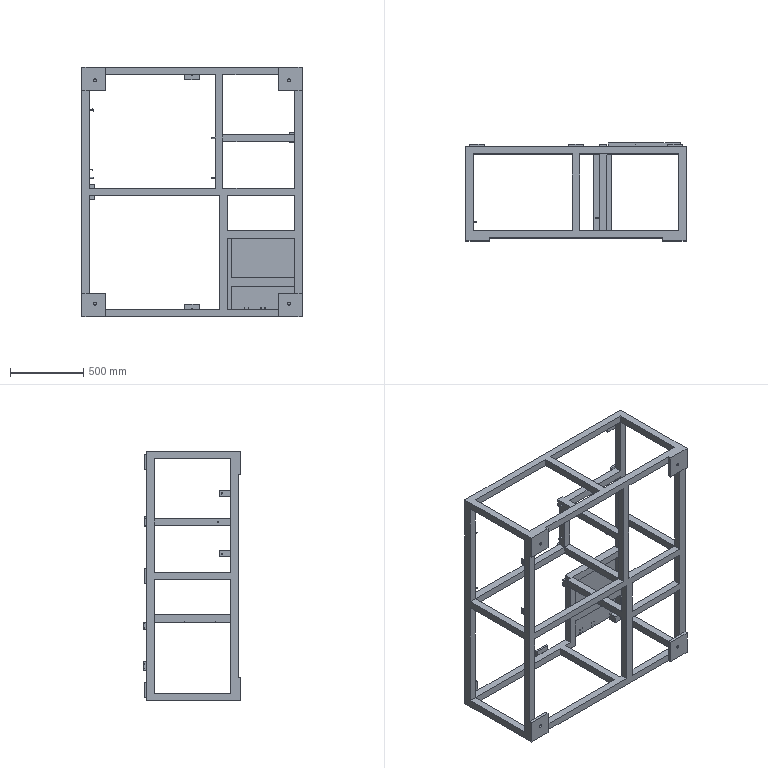Part | STEP file | 11-FG-JX00211 | 1 solid | 604 faces | box 1500 x 667.5 x 1700 mm | volume 66450953 mm3 | cylinder 228 | plane 192 | cone 184 | commonest cylinder face diameters 3.3 x74 4.2 x60 5 x40 6.8 x32 8 x14 21 x8